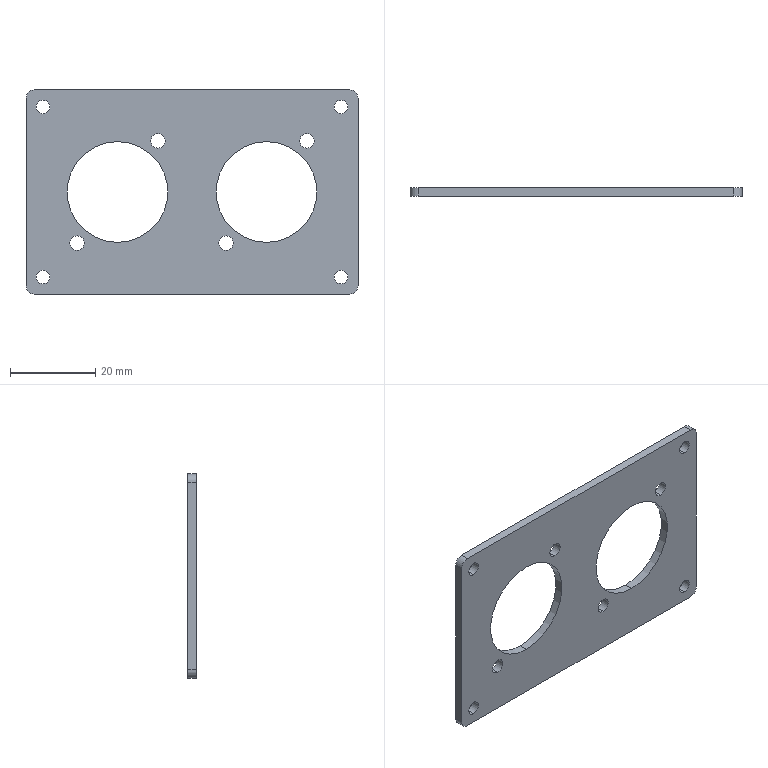Part | SolidWorks | features MoveFace 2, Cut 1, Extrusion 1, Fillet 1, ICE 1, LPattern 1 | 1 solid | 153 faces | box 78 x 2 x 48 mm | volume 5579 mm3 | plane 78 | spline 51 | cylinder 24 | commonest cylinder face diameters 3.2 x8 3.4 x8 4 x4 23.7 x4